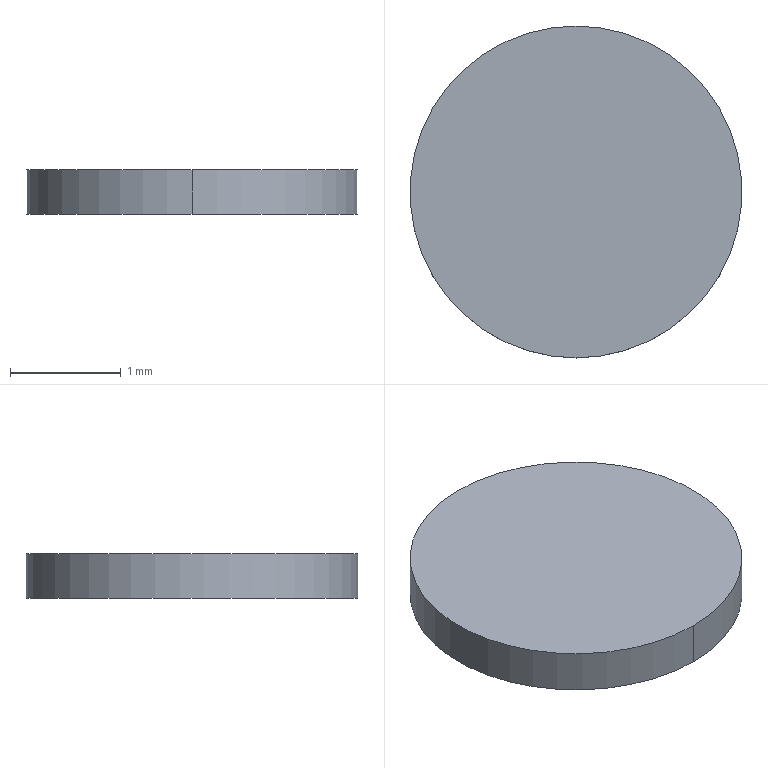Part | STEP file | LRS-150-12_X2_5F00517375-151335 | 1 solid | 4 faces | box 3 x 3 x 0.4 mm | volume 2.827 mm3 | cylinder 2 | plane 2 | commonest cylinder face diameters 3 x2
STEP:
#1=CARTESIAN_POINT('',(0.,0.,0.));
#2=DIRECTION('',(0.,0.,1.));
#3=DIRECTION('',(1.,0.,0.));
#4=AXIS2_PLACEMENT_3D('',#1,#2,#3);
#5=CARTESIAN_POINT('',(-271.167,263.625,-4.4));
#6=VERTEX_POINT('',#5);
#7=CARTESIAN_POINT('',(-271.167,263.625,-4.8));
#8=VERTEX_POINT('',#7);
#9=CARTESIAN_POINT('',(-271.167,263.625,-4.4));
#10=DIRECTION('',(0.,0.,-1.));
#11=VECTOR('',#10,1.);
#12=LINE('',#9,#11);
#13=CARTESIAN_POINT('',(-271.167,265.125,-1.6));
#14=DIRECTION('',(0.,0.,-1.));
#15=DIRECTION('',(0.,1.,0.));
#16=AXIS2_PLACEMENT_3D('',#13,#14,#15);
#17=CYLINDRICAL_SURFACE('',#16,1.5);
#18=CARTESIAN_POINT('',(3.142,2.8));
#19=DIRECTION('',(0.,1.));
#20=VECTOR('',#19,1.);
#21=LINE('',#18,#20);
#22=(GEOMETRIC_REPRESENTATION_CONTEXT(2)PARAMETRIC_REPRESENTATION_CONTEXT()REPRESENTATION_CONTEXT('',''));
#23=DEFINITIONAL_REPRESENTATION('',(#21),#22);
#24=PCURVE('',#17,#23);
#25=CARTESIAN_POINT('',(-271.167,265.125,-1.6));
#26=DIRECTION('',(0.,0.,-1.));
#27=DIRECTION('',(0.,1.,0.));
#28=AXIS2_PLACEMENT_3D('',#25,#26,#27);
#29=CYLINDRICAL_SURFACE('',#28,1.5);
#30=CARTESIAN_POINT('',(3.142,2.8));
#31=DIRECTION('',(0.,1.));
#32=VECTOR('',#31,1.);
#33=LINE('',#30,#32);
#34=(GEOMETRIC_REPRESENTATION_CONTEXT(2)PARAMETRIC_REPRESENTATION_CONTEXT()REPRESENTATION_CONTEXT('',''));
#35=DEFINITIONAL_REPRESENTATION('',(#33),#34);
#36=PCURVE('',#29,#35);
#37=SURFACE_CURVE('',#12,(#24,#36),.PCURVE_S1.);
#38=EDGE_CURVE('',#6,#8,#37,.T.);
#39=ORIENTED_EDGE('',*,*,#38,.F.);
#40=CARTESIAN_POINT('',(-271.167,266.625,-4.4));
#41=VERTEX_POINT('',#40);
#42=CARTESIAN_POINT('',(-271.167,265.125,-4.4));
#43=DIRECTION('',(0.,0.,1.));
#44=DIRECTION('',(0.,1.,0.));
#45=AXIS2_PLACEMENT_3D('',#42,#43,#44);
#46=CIRCLE('',#45,1.5);
#47=CARTESIAN_POINT('',(6.283,2.8));
#48=DIRECTION('',(-1.,0.));
#49=VECTOR('',#48,1.);
#50=LINE('',#47,#49);
#51=(GEOMETRIC_REPRESENTATION_CONTEXT(2)PARAMETRIC_REPRESENTATION_CONTEXT()REPRESENTATION_CONTEXT('',''));
#52=DEFINITIONAL_REPRESENTATION('',(#50),#51);
#53=PCURVE('',#17,#52);
#54=CARTESIAN_POINT('',(-217.675,251.825,-4.4));
#55=DIRECTION('',(0.,0.,-1.));
#56=DIRECTION('',(1.,0.,0.));
#57=AXIS2_PLACEMENT_3D('',#54,#55,#56);
#58=PLANE('',#57);
#59=CARTESIAN_POINT('',(-53.491,-14.8));
#60=CARTESIAN_POINT('',(-56.089,-14.8));
#61=CARTESIAN_POINT('',(-54.79,-12.55));
#62=CARTESIAN_POINT('',(-53.491,-10.3));
#63=CARTESIAN_POINT('',(-52.192,-12.55));
#64=CARTESIAN_POINT('',(-50.893,-14.8));
#65=CARTESIAN_POINT('',(-53.491,-14.8));
#66=(BOUNDED_CURVE()B_SPLINE_CURVE(2,(#59,#60,#61,#62,#63,#64,#65),.UNSPECIFIED.,.T.,.F.)B_SPLINE_CURVE_WITH_KNOTS((1,2,2,2,2,1),(-2.094,0.,2.094,4.189,6.283,8.378),.UNSPECIFIED.)CURVE()GEOMETRIC_REPRESENTATION_ITEM()RATIONAL_B_SPLINE_CURVE((1.,0.5,1.,0.5,1.,0.5,1.))REPRESENTATION_ITEM(''));
#67=(GEOMETRIC_REPRESENTATION_CONTEXT(2)PARAMETRIC_REPRESENTATION_CONTEXT()REPRESENTATION_CONTEXT('',''));
#68=DEFINITIONAL_REPRESENTATION('',(#66),#67);
#69=PCURVE('',#58,#68);
#70=SURFACE_CURVE('',#46,(#53,#69),.PCURVE_S1.);
#71=EDGE_CURVE('',#41,#6,#70,.T.);
#72=ORIENTED_EDGE('',*,*,#71,.F.);
#73=CARTESIAN_POINT('',(-271.167,266.625,-4.8));
#74=VERTEX_POINT('',#73);
#75=CARTESIAN_POINT('',(-271.167,266.625,-4.4));
#76=DIRECTION('',(0.,0.,-1.));
#77=VECTOR('',#76,1.);
#78=LINE('',#75,#77);
#79=CARTESIAN_POINT('',(6.283,2.8));
#80=DIRECTION('',(0.,1.));
#81=VECTOR('',#80,1.);
#82=LINE('',#79,#81);
#83=(GEOMETRIC_REPRESENTATION_CONTEXT(2)PARAMETRIC_REPRESENTATION_CONTEXT()REPRESENTATION_CONTEXT('',''));
#84=DEFINITIONAL_REPRESENTATION('',(#82),#83);
#85=PCURVE('',#17,#84);
#86=CARTESIAN_POINT('',(0.,2.8));
#87=DIRECTION('',(0.,1.));
#88=VECTOR('',#87,1.);
#89=LINE('',#86,#88);
#90=(GEOMETRIC_REPRESENTATION_CONTEXT(2)PARAMETRIC_REPRESENTATION_CONTEXT()REPRESENTATION_CONTEXT('',''));
#91=DEFINITIONAL_REPRESENTATION('',(#89),#90);
#92=PCURVE('',#29,#91);
#93=SURFACE_CURVE('',#78,(#85,#92),.PCURVE_S1.);
#94=EDGE_CURVE('',#41,#74,#93,.T.);
#95=ORIENTED_EDGE('',*,*,#94,.T.);
#96=CARTESIAN_POINT('',(-271.167,265.125,-4.8));
#97=DIRECTION('',(0.,0.,-1.));
#98=DIRECTION('',(0.,-1.,0.));
#99=AXIS2_PLACEMENT_3D('',#96,#97,#98);
#100=CIRCLE('',#99,1.5);
#101=CARTESIAN_POINT('',(3.142,3.2));
#102=DIRECTION('',(1.,0.));
#103=VECTOR('',#102,1.);
#104=LINE('',#101,#103);
#105=(GEOMETRIC_REPRESENTATION_CONTEXT(2)PARAMETRIC_REPRESENTATION_CONTEXT()REPRESENTATION_CONTEXT('',''));
#106=DEFINITIONAL_REPRESENTATION('',(#104),#105);
#107=PCURVE('',#17,#106);
#108=CARTESIAN_POINT('',(-217.675,251.825,-4.8));
#109=DIRECTION('',(0.,0.,-1.));
#110=DIRECTION('',(1.,0.,0.));
#111=AXIS2_PLACEMENT_3D('',#108,#109,#110);
#112=PLANE('',#111);
#113=CARTESIAN_POINT('',(-53.491,-13.3));
#114=DIRECTION('',(0.,1.));
#115=AXIS2_PLACEMENT_2D('',#113,#114);
#116=CIRCLE('',#115,1.5);
#117=(GEOMETRIC_REPRESENTATION_CONTEXT(2)PARAMETRIC_REPRESENTATION_CONTEXT()REPRESENTATION_CONTEXT('',''));
#118=DEFINITIONAL_REPRESENTATION('',(#116),#117);
#119=PCURVE('',#112,#118);
#120=SURFACE_CURVE('',#100,(#107,#119),.PCURVE_S1.);
#121=EDGE_CURVE('',#8,#74,#120,.T.);
#122=ORIENTED_EDGE('',*,*,#121,.F.);
#123=EDGE_LOOP('',(#39,#72,#95,#122));
#124=FACE_BOUND('',#123,.T.);
#125=ADVANCED_FACE('',(#124),#17,.T.);
#126=ORIENTED_EDGE('',*,*,#121,.F.);
#127=CARTESIAN_POINT('',(-271.167,265.125,-4.8));
#128=DIRECTION('',(0.,0.,-1.));
#129=DIRECTION('',(0.,1.,0.));
#130=AXIS2_PLACEMENT_3D('',#127,#128,#129);
#131=CIRCLE('',#130,1.5);
#132=CARTESIAN_POINT('',(-53.491,-13.3));
#133=DIRECTION('',(0.,-1.));
#134=AXIS2_PLACEMENT_2D('',#132,#133);
#135=CIRCLE('',#134,1.5);
#136=(GEOMETRIC_REPRESENTATION_CONTEXT(2)PARAMETRIC_REPRESENTATION_CONTEXT()REPRESENTATION_CONTEXT('',''));
#137=DEFINITIONAL_REPRESENTATION('',(#135),#136);
#138=PCURVE('',#112,#137);
#139=CARTESIAN_POINT('',(0.,3.2));
#140=DIRECTION('',(1.,0.));
#141=VECTOR('',#140,1.);
#142=LINE('',#139,#141);
#143=(GEOMETRIC_REPRESENTATION_CONTEXT(2)PARAMETRIC_REPRESENTATION_CONTEXT()REPRESENTATION_CONTEXT('',''));
#144=DEFINITIONAL_REPRESENTATION('',(#142),#143);
#145=PCURVE('',#29,#144);
#146=SURFACE_CURVE('',#131,(#138,#145),.PCURVE_S1.);
#147=EDGE_CURVE('',#74,#8,#146,.T.);
#148=ORIENTED_EDGE('',*,*,#147,.F.);
#149=EDGE_LOOP('',(#126,#148));
#150=FACE_BOUND('',#149,.F.);
#151=ADVANCED_FACE('',(#150),#112,.T.);
#152=ORIENTED_EDGE('',*,*,#147,.F.);
#153=ORIENTED_EDGE('',*,*,#94,.F.);
#154=CARTESIAN_POINT('',(-271.167,265.125,-4.4));
#155=DIRECTION('',(0.,0.,1.));
#156=DIRECTION('',(0.,-1.,0.));
#157=AXIS2_PLACEMENT_3D('',#154,#155,#156);
#158=CIRCLE('',#157,1.5);
#159=CARTESIAN_POINT('',(3.142,2.8));
#160=DIRECTION('',(-1.,0.));
#161=VECTOR('',#160,1.);
#162=LINE('',#159,#161);
#163=(GEOMETRIC_REPRESENTATION_CONTEXT(2)PARAMETRIC_REPRESENTATION_CONTEXT()REPRESENTATION_CONTEXT('',''));
#164=DEFINITIONAL_REPRESENTATION('',(#162),#163);
#165=PCURVE('',#29,#164);
#166=CARTESIAN_POINT('',(-53.491,-11.8));
#167=CARTESIAN_POINT('',(-50.893,-11.8));
#168=CARTESIAN_POINT('',(-52.192,-14.05));
#169=CARTESIAN_POINT('',(-53.491,-16.3));
#170=CARTESIAN_POINT('',(-54.79,-14.05));
#171=CARTESIAN_POINT('',(-56.089,-11.8));
#172=CARTESIAN_POINT('',(-53.491,-11.8));
#173=(BOUNDED_CURVE()B_SPLINE_CURVE(2,(#166,#167,#168,#169,#170,#171,#172),.UNSPECIFIED.,.T.,.F.)B_SPLINE_CURVE_WITH_KNOTS((1,2,2,2,2,1),(-2.094,0.,2.094,4.189,6.283,8.378),.UNSPECIFIED.)CURVE()GEOMETRIC_REPRESENTATION_ITEM()RATIONAL_B_SPLINE_CURVE((1.,0.5,1.,0.5,1.,0.5,1.))REPRESENTATION_ITEM(''));
#174=(GEOMETRIC_REPRESENTATION_CONTEXT(2)PARAMETRIC_REPRESENTATION_CONTEXT()REPRESENTATION_CONTEXT('',''));
#175=DEFINITIONAL_REPRESENTATION('',(#173),#174);
#176=PCURVE('',#58,#175);
#177=SURFACE_CURVE('',#158,(#165,#176),.PCURVE_S1.);
#178=EDGE_CURVE('',#6,#41,#177,.T.);
#179=ORIENTED_EDGE('',*,*,#178,.F.);
#180=ORIENTED_EDGE('',*,*,#38,.T.);
#181=EDGE_LOOP('',(#152,#153,#179,#180));
#182=FACE_BOUND('',#181,.T.);
#183=ADVANCED_FACE('',(#182),#29,.T.);
#184=ORIENTED_EDGE('',*,*,#71,.F.);
#185=ORIENTED_EDGE('',*,*,#178,.F.);
#186=EDGE_LOOP('',(#184,#185));
#187=FACE_BOUND('',#186,.F.);
#188=ADVANCED_FACE('',(#187),#58,.F.);
#189=CLOSED_SHELL('',(#125,#151,#183,#188));
#190=MANIFOLD_SOLID_BREP('',#189);
#191=(LENGTH_UNIT()NAMED_UNIT(*)SI_UNIT(.MILLI.,.METRE.));
#192=UNCERTAINTY_MEASURE_WITH_UNIT(LENGTH_MEASURE(0.0000001),#191,'','');
#193=(NAMED_UNIT(*)PLANE_ANGLE_UNIT()SI_UNIT($,.RADIAN.));
#194=(NAMED_UNIT(*)SI_UNIT($,.STERADIAN.)SOLID_ANGLE_UNIT());
#195=(GEOMETRIC_REPRESENTATION_CONTEXT(3)GLOBAL_UNCERTAINTY_ASSIGNED_CONTEXT((#192))GLOBAL_UNIT_ASSIGNED_CONTEXT((#191,#193,#194))REPRESENTATION_CONTEXT('',''));
#196=ADVANCED_BREP_SHAPE_REPRESENTATION('',(#4,#190),#195);